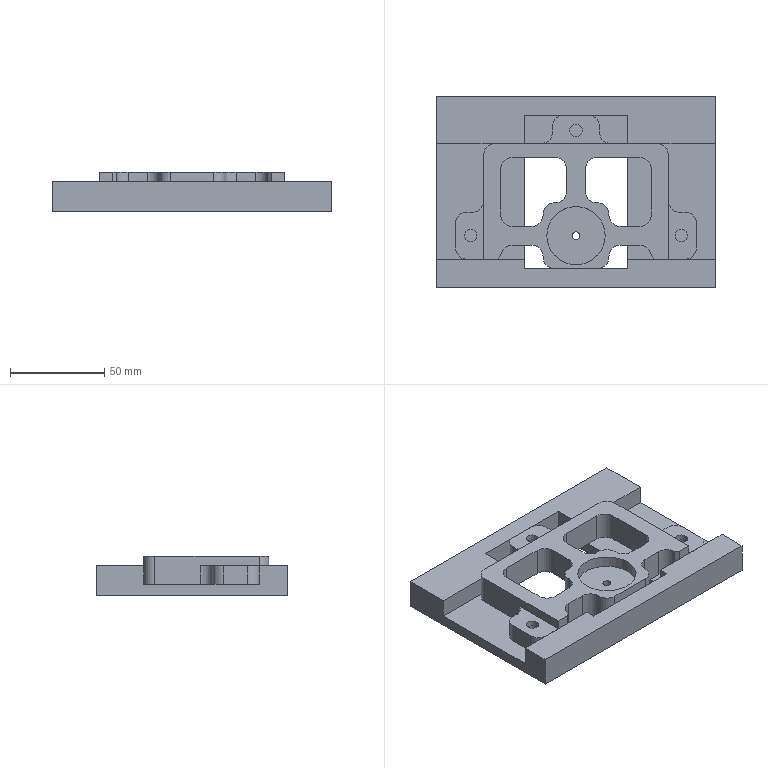Part | 2 solids | 99 faces | box 148 x 101.5 x 21 mm | volume 177433 mm3 | plane 60 | cylinder 39 | commonest cylinder face diameters 12 x30 6.6 x3 11 x3 4.2 x1 30.6 x1 31 x1